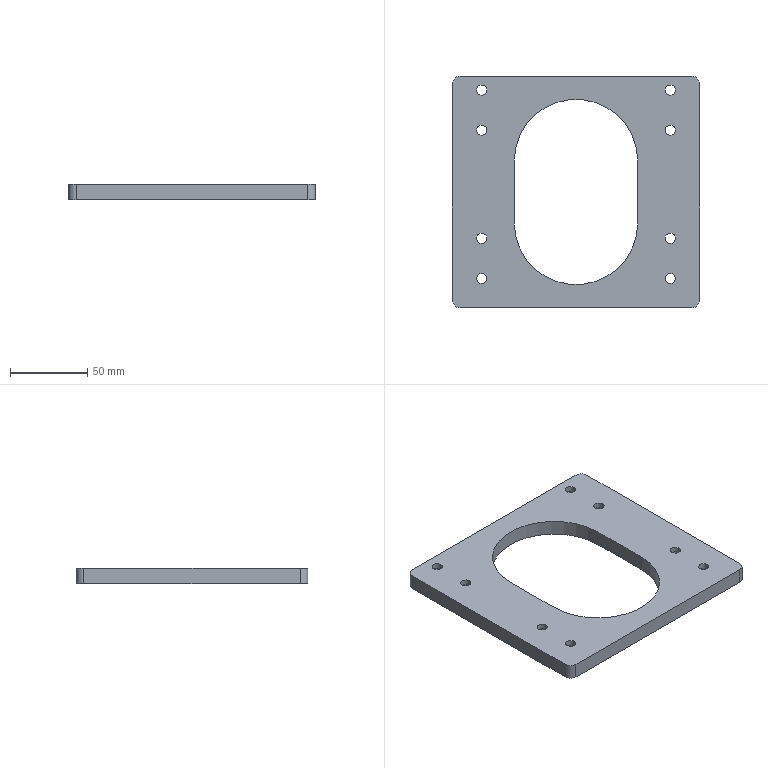Part | SolidWorks | features Cut 1, Extrusion 1, Fillet 1, HoleWzd 1 | 1 solid | 54 faces | box 160 x 150 x 10 mm | volume 151669 mm3 | cylinder 38 | plane 16 | commonest cylinder face diameters 6.6 x16 11 x16 10 x4 80 x2